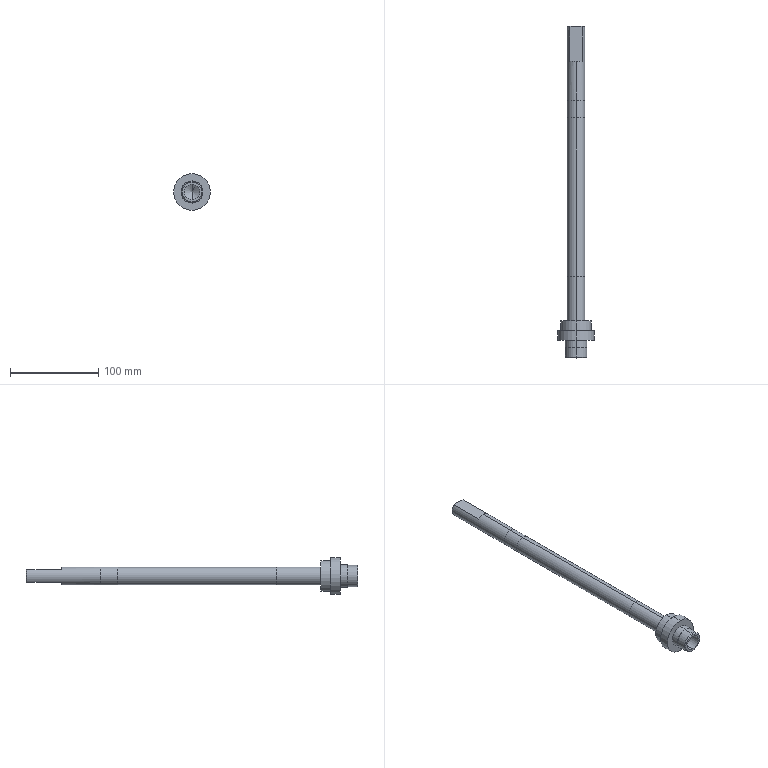Part | SolidWorks | features BaseBody 2 | 2 solids | 38 faces | box 41.4 x 376 x 41.4 mm | volume 127294 mm3 | cylinder 18 | plane 14 | cone 6 | commonest cylinder face diameters 20 x6 17.5 x2 19.8 x2 24 x2 25 x2 35 x2
STEP:
#1=CARTESIAN_POINT('',(7.141,244.,7.));
#2=VERTEX_POINT('',#1);
#3=CARTESIAN_POINT('',(0.,244.,10.));
#4=VERTEX_POINT('',#3);
#5=CARTESIAN_POINT('',(0.,244.,0.));
#6=DIRECTION('',(0.,-1.,0.));
#7=DIRECTION('',(0.,0.,-1.));
#8=AXIS2_PLACEMENT_3D('',#5,#6,#7);
#9=CIRCLE('',#8,10.);
#10=EDGE_CURVE('',#2,#4,#9,.T.);
#11=ORIENTED_EDGE('',*,*,#10,.T.);
#12=CARTESIAN_POINT('',(0.,200.,10.));
#13=VERTEX_POINT('',#12);
#14=CARTESIAN_POINT('',(0.,284.,10.));
#15=DIRECTION('',(0.,-1.,0.));
#16=VECTOR('',#15,1000.);
#17=LINE('',#14,#16);
#18=EDGE_CURVE('',#4,#13,#17,.T.);
#19=ORIENTED_EDGE('',*,*,#18,.T.);
#20=CARTESIAN_POINT('',(0.,200.,-10.));
#21=VERTEX_POINT('',#20);
#22=CARTESIAN_POINT('',(0.,200.,0.));
#23=DIRECTION('',(0.,1.,0.));
#24=DIRECTION('',(0.,0.,-1.));
#25=AXIS2_PLACEMENT_3D('',#22,#23,#24);
#26=CIRCLE('',#25,10.);
#27=EDGE_CURVE('',#13,#21,#26,.T.);
#28=ORIENTED_EDGE('',*,*,#27,.T.);
#29=CARTESIAN_POINT('',(0.,244.,-10.));
#30=VERTEX_POINT('',#29);
#31=CARTESIAN_POINT('',(0.,284.,-10.));
#32=DIRECTION('',(0.,-1.,0.));
#33=VECTOR('',#32,1000.);
#34=LINE('',#31,#33);
#35=EDGE_CURVE('',#30,#21,#34,.T.);
#36=ORIENTED_EDGE('',*,*,#35,.F.);
#37=CARTESIAN_POINT('',(7.141,244.,-7.));
#38=VERTEX_POINT('',#37);
#39=CARTESIAN_POINT('',(0.,244.,0.));
#40=DIRECTION('',(0.,-1.,0.));
#41=DIRECTION('',(0.,0.,-1.));
#42=AXIS2_PLACEMENT_3D('',#39,#40,#41);
#43=CIRCLE('',#42,10.);
#44=EDGE_CURVE('',#30,#38,#43,.T.);
#45=ORIENTED_EDGE('',*,*,#44,.T.);
#46=CARTESIAN_POINT('',(7.141,283.,-7.));
#47=VERTEX_POINT('',#46);
#48=CARTESIAN_POINT('',(7.141,284.,-7.));
#49=DIRECTION('',(0.,1.,0.));
#50=VECTOR('',#49,1000.);
#51=LINE('',#48,#50);
#52=EDGE_CURVE('',#38,#47,#51,.T.);
#53=ORIENTED_EDGE('',*,*,#52,.T.);
#54=CARTESIAN_POINT('',(7.141,283.,7.));
#55=VERTEX_POINT('',#54);
#56=CARTESIAN_POINT('',(0.,283.,0.));
#57=DIRECTION('',(0.,-1.,0.));
#58=DIRECTION('',(0.,0.,-1.));
#59=AXIS2_PLACEMENT_3D('',#56,#57,#58);
#60=CIRCLE('',#59,10.);
#61=EDGE_CURVE('',#47,#55,#60,.T.);
#62=ORIENTED_EDGE('',*,*,#61,.T.);
#63=CARTESIAN_POINT('',(7.141,284.,7.));
#64=DIRECTION('',(0.,-1.,0.));
#65=VECTOR('',#64,1000.);
#66=LINE('',#63,#65);
#67=EDGE_CURVE('',#55,#2,#66,.T.);
#68=ORIENTED_EDGE('',*,*,#67,.T.);
#69=EDGE_LOOP('',(#11,#19,#28,#36,#45,#53,#62,#68));
#70=FACE_OUTER_BOUND('',#69,.T.);
#71=CARTESIAN_POINT('',(0.,284.,0.));
#72=DIRECTION('',(0.,-1.,0.));
#73=DIRECTION('',(0.,0.,-1.));
#74=AXIS2_PLACEMENT_3D('',#71,#72,#73);
#75=CYLINDRICAL_SURFACE('',#74,10.);
#76=ADVANCED_FACE('',(#70),#75,.T.);
#77=ORIENTED_EDGE('',*,*,#18,.F.);
#78=CARTESIAN_POINT('',(-7.141,244.,7.));
#79=VERTEX_POINT('',#78);
#80=CARTESIAN_POINT('',(0.,244.,0.));
#81=DIRECTION('',(0.,-1.,0.));
#82=DIRECTION('',(0.,0.,-1.));
#83=AXIS2_PLACEMENT_3D('',#80,#81,#82);
#84=CIRCLE('',#83,10.);
#85=EDGE_CURVE('',#4,#79,#84,.T.);
#86=ORIENTED_EDGE('',*,*,#85,.T.);
#87=CARTESIAN_POINT('',(-7.141,283.,7.));
#88=VERTEX_POINT('',#87);
#89=CARTESIAN_POINT('',(-7.141,244.,7.));
#90=DIRECTION('',(0.,-1.,0.));
#91=VECTOR('',#90,1000.);
#92=LINE('',#89,#91);
#93=EDGE_CURVE('',#88,#79,#92,.T.);
#94=ORIENTED_EDGE('',*,*,#93,.F.);
#95=CARTESIAN_POINT('',(-7.141,283.,-7.));
#96=VERTEX_POINT('',#95);
#97=CARTESIAN_POINT('',(0.,283.,0.));
#98=DIRECTION('',(0.,-1.,0.));
#99=DIRECTION('',(0.,0.,-1.));
#100=AXIS2_PLACEMENT_3D('',#97,#98,#99);
#101=CIRCLE('',#100,10.);
#102=EDGE_CURVE('',#88,#96,#101,.T.);
#103=ORIENTED_EDGE('',*,*,#102,.T.);
#104=CARTESIAN_POINT('',(-7.141,244.,-7.));
#105=VERTEX_POINT('',#104);
#106=CARTESIAN_POINT('',(-7.141,244.,-7.));
#107=DIRECTION('',(0.,1.,0.));
#108=VECTOR('',#107,1000.);
#109=LINE('',#106,#108);
#110=EDGE_CURVE('',#105,#96,#109,.T.);
#111=ORIENTED_EDGE('',*,*,#110,.F.);
#112=CARTESIAN_POINT('',(0.,244.,0.));
#113=DIRECTION('',(0.,-1.,0.));
#114=DIRECTION('',(0.,0.,-1.));
#115=AXIS2_PLACEMENT_3D('',#112,#113,#114);
#116=CIRCLE('',#115,10.);
#117=EDGE_CURVE('',#105,#30,#116,.T.);
#118=ORIENTED_EDGE('',*,*,#117,.T.);
#119=ORIENTED_EDGE('',*,*,#35,.T.);
#120=CARTESIAN_POINT('',(0.,200.,0.));
#121=DIRECTION('',(0.,1.,0.));
#122=DIRECTION('',(0.,0.,-1.));
#123=AXIS2_PLACEMENT_3D('',#120,#121,#122);
#124=CIRCLE('',#123,10.);
#125=EDGE_CURVE('',#21,#13,#124,.T.);
#126=ORIENTED_EDGE('',*,*,#125,.T.);
#127=EDGE_LOOP('',(#77,#86,#94,#103,#111,#118,#119,#126));
#128=FACE_OUTER_BOUND('',#127,.T.);
#129=CARTESIAN_POINT('',(0.,284.,0.));
#130=DIRECTION('',(0.,-1.,0.));
#131=DIRECTION('',(0.,0.,-1.));
#132=AXIS2_PLACEMENT_3D('',#129,#130,#131);
#133=CYLINDRICAL_SURFACE('',#132,10.);
#134=ADVANCED_FACE('',(#128),#133,.T.);
#135=ORIENTED_EDGE('',*,*,#93,.T.);
#136=CARTESIAN_POINT('',(-15.568,244.,7.));
#137=DIRECTION('',(1.,0.,0.));
#138=VECTOR('',#137,1000.);
#139=LINE('',#136,#138);
#140=EDGE_CURVE('',#79,#2,#139,.T.);
#141=ORIENTED_EDGE('',*,*,#140,.T.);
#142=ORIENTED_EDGE('',*,*,#67,.F.);
#143=CARTESIAN_POINT('',(5.657,284.,7.));
#144=VERTEX_POINT('',#143);
#145=CARTESIAN_POINT('',(7.141,283.,7.));
#146=CARTESIAN_POINT('',(6.656,283.347,7.));
#147=CARTESIAN_POINT('',(6.162,283.682,7.));
#148=CARTESIAN_POINT('',(5.657,284.,7.));
#149=B_SPLINE_CURVE_WITH_KNOTS('',3,(#145,#146,#147,#148),.UNSPECIFIED.,.F.,.F.,(4,4),(0.,0.00179),.UNSPECIFIED.);
#150=EDGE_CURVE('',#55,#144,#149,.T.);
#151=ORIENTED_EDGE('',*,*,#150,.T.);
#152=CARTESIAN_POINT('',(-5.657,284.,7.));
#153=VERTEX_POINT('',#152);
#154=CARTESIAN_POINT('',(-15.568,284.,7.));
#155=DIRECTION('',(-1.,0.,0.));
#156=VECTOR('',#155,1000.);
#157=LINE('',#154,#156);
#158=EDGE_CURVE('',#144,#153,#157,.T.);
#159=ORIENTED_EDGE('',*,*,#158,.T.);
#160=CARTESIAN_POINT('',(-5.657,284.,7.));
#161=CARTESIAN_POINT('',(-6.162,283.682,7.));
#162=CARTESIAN_POINT('',(-6.656,283.347,7.));
#163=CARTESIAN_POINT('',(-7.141,283.,7.));
#164=B_SPLINE_CURVE_WITH_KNOTS('',3,(#160,#161,#162,#163),.UNSPECIFIED.,.F.,.F.,(4,4),(0.,0.00179),.UNSPECIFIED.);
#165=EDGE_CURVE('',#153,#88,#164,.T.);
#166=ORIENTED_EDGE('',*,*,#165,.T.);
#167=EDGE_LOOP('',(#135,#141,#142,#151,#159,#166));
#168=FACE_OUTER_BOUND('',#167,.T.);
#169=CARTESIAN_POINT('',(-15.568,244.,7.));
#170=DIRECTION('',(0.,0.,1.));
#171=DIRECTION('',(1.,0.,0.));
#172=AXIS2_PLACEMENT_3D('',#169,#170,#171);
#173=PLANE('',#172);
#174=ADVANCED_FACE('',(#168),#173,.T.);
#175=CARTESIAN_POINT('',(5.657,284.,-7.));
#176=VERTEX_POINT('',#175);
#177=CARTESIAN_POINT('',(7.141,283.,-7.));
#178=CARTESIAN_POINT('',(6.656,283.347,-7.));
#179=CARTESIAN_POINT('',(6.162,283.682,-7.));
#180=CARTESIAN_POINT('',(5.657,284.,-7.));
#181=B_SPLINE_CURVE_WITH_KNOTS('',3,(#177,#178,#179,#180),.UNSPECIFIED.,.F.,.F.,(4,4),(0.,0.00179),.UNSPECIFIED.);
#182=EDGE_CURVE('',#47,#176,#181,.T.);
#183=ORIENTED_EDGE('',*,*,#182,.T.);
#184=CARTESIAN_POINT('',(0.,284.,0.));
#185=DIRECTION('',(0.,-1.,0.));
#186=DIRECTION('',(0.,0.,-1.));
#187=AXIS2_PLACEMENT_3D('',#184,#185,#186);
#188=CIRCLE('',#187,9.);
#189=EDGE_CURVE('',#176,#144,#188,.T.);
#190=ORIENTED_EDGE('',*,*,#189,.T.);
#191=ORIENTED_EDGE('',*,*,#150,.F.);
#192=ORIENTED_EDGE('',*,*,#61,.F.);
#193=EDGE_LOOP('',(#183,#190,#191,#192));
#194=FACE_OUTER_BOUND('',#193,.T.);
#195=CARTESIAN_POINT('',(0.,283.,0.));
#196=DIRECTION('',(0.,-1.,0.));
#197=DIRECTION('',(0.,0.,-1.));
#198=AXIS2_PLACEMENT_3D('',#195,#196,#197);
#199=CONICAL_SURFACE('',#198,10.,0.7854);
#200=ADVANCED_FACE('',(#194),#199,.T.);
#201=ORIENTED_EDGE('',*,*,#110,.T.);
#202=CARTESIAN_POINT('',(-5.657,284.,-7.));
#203=VERTEX_POINT('',#202);
#204=CARTESIAN_POINT('',(-7.141,283.,-7.));
#205=CARTESIAN_POINT('',(-6.656,283.347,-7.));
#206=CARTESIAN_POINT('',(-6.162,283.682,-7.));
#207=CARTESIAN_POINT('',(-5.657,284.,-7.));
#208=B_SPLINE_CURVE_WITH_KNOTS('',3,(#204,#205,#206,#207),.UNSPECIFIED.,.F.,.F.,(4,4),(0.,0.00179),.UNSPECIFIED.);
#209=EDGE_CURVE('',#96,#203,#208,.T.);
#210=ORIENTED_EDGE('',*,*,#209,.T.);
#211=CARTESIAN_POINT('',(-15.568,284.,-7.));
#212=DIRECTION('',(1.,0.,0.));
#213=VECTOR('',#212,1000.);
#214=LINE('',#211,#213);
#215=EDGE_CURVE('',#203,#176,#214,.T.);
#216=ORIENTED_EDGE('',*,*,#215,.T.);
#217=ORIENTED_EDGE('',*,*,#182,.F.);
#218=ORIENTED_EDGE('',*,*,#52,.F.);
#219=CARTESIAN_POINT('',(-15.568,244.,-7.));
#220=DIRECTION('',(-1.,0.,0.));
#221=VECTOR('',#220,1000.);
#222=LINE('',#219,#221);
#223=EDGE_CURVE('',#38,#105,#222,.T.);
#224=ORIENTED_EDGE('',*,*,#223,.T.);
#225=EDGE_LOOP('',(#201,#210,#216,#217,#218,#224));
#226=FACE_OUTER_BOUND('',#225,.T.);
#227=CARTESIAN_POINT('',(-15.568,244.,-7.));
#228=DIRECTION('',(0.,0.,-1.));
#229=DIRECTION('',(-1.,0.,0.));
#230=AXIS2_PLACEMENT_3D('',#227,#228,#229);
#231=PLANE('',#230);
#232=ADVANCED_FACE('',(#226),#231,.T.);
#233=ORIENTED_EDGE('',*,*,#117,.F.);
#234=ORIENTED_EDGE('',*,*,#223,.F.);
#235=ORIENTED_EDGE('',*,*,#44,.F.);
#236=EDGE_LOOP('',(#233,#234,#235));
#237=FACE_OUTER_BOUND('',#236,.T.);
#238=CARTESIAN_POINT('',(0.,244.,0.));
#239=DIRECTION('',(0.,1.,0.));
#240=DIRECTION('',(0.,0.,1.));
#241=AXIS2_PLACEMENT_3D('',#238,#239,#240);
#242=PLANE('',#241);
#243=ADVANCED_FACE('',(#237),#242,.T.);
#244=ORIENTED_EDGE('',*,*,#125,.F.);
#245=ORIENTED_EDGE('',*,*,#27,.F.);
#246=EDGE_LOOP('',(#244,#245));
#247=FACE_OUTER_BOUND('',#246,.T.);
#248=CARTESIAN_POINT('',(0.,200.,0.));
#249=DIRECTION('',(0.,1.,0.));
#250=DIRECTION('',(0.,0.,1.));
#251=AXIS2_PLACEMENT_3D('',#248,#249,#250);
#252=PLANE('',#251);
#253=ADVANCED_FACE('',(#247),#252,.F.);
#254=ORIENTED_EDGE('',*,*,#10,.F.);
#255=ORIENTED_EDGE('',*,*,#140,.F.);
#256=ORIENTED_EDGE('',*,*,#85,.F.);
#257=EDGE_LOOP('',(#254,#255,#256));
#258=FACE_OUTER_BOUND('',#257,.T.);
#259=CARTESIAN_POINT('',(0.,244.,0.));
#260=DIRECTION('',(0.,1.,0.));
#261=DIRECTION('',(0.,0.,1.));
#262=AXIS2_PLACEMENT_3D('',#259,#260,#261);
#263=PLANE('',#262);
#264=ADVANCED_FACE('',(#258),#263,.T.);
#265=ORIENTED_EDGE('',*,*,#165,.F.);
#266=CARTESIAN_POINT('',(0.,284.,0.));
#267=DIRECTION('',(0.,-1.,0.));
#268=DIRECTION('',(0.,0.,-1.));
#269=AXIS2_PLACEMENT_3D('',#266,#267,#268);
#270=CIRCLE('',#269,9.);
#271=EDGE_CURVE('',#153,#203,#270,.T.);
#272=ORIENTED_EDGE('',*,*,#271,.T.);
#273=ORIENTED_EDGE('',*,*,#209,.F.);
#274=ORIENTED_EDGE('',*,*,#102,.F.);
#275=EDGE_LOOP('',(#265,#272,#273,#274));
#276=FACE_OUTER_BOUND('',#275,.T.);
#277=CARTESIAN_POINT('',(0.,283.,0.));
#278=DIRECTION('',(0.,-1.,0.));
#279=DIRECTION('',(0.,0.,-1.));
#280=AXIS2_PLACEMENT_3D('',#277,#278,#279);
#281=CONICAL_SURFACE('',#280,10.,0.7854);
#282=ADVANCED_FACE('',(#276),#281,.T.);
#283=ORIENTED_EDGE('',*,*,#215,.F.);
#284=ORIENTED_EDGE('',*,*,#271,.F.);
#285=ORIENTED_EDGE('',*,*,#158,.F.);
#286=ORIENTED_EDGE('',*,*,#189,.F.);
#287=EDGE_LOOP('',(#283,#284,#285,#286));
#288=FACE_OUTER_BOUND('',#287,.T.);
#289=CARTESIAN_POINT('',(0.,284.,0.));
#290=DIRECTION('',(0.,1.,0.));
#291=DIRECTION('',(0.,0.,1.));
#292=AXIS2_PLACEMENT_3D('',#289,#290,#291);
#293=PLANE('',#292);
#294=ADVANCED_FACE('',(#288),#293,.T.);
#295=CLOSED_SHELL('',(#76,#134,#174,#200,#232,#243,#253,#264,#282,#294));
#296=MANIFOLD_SOLID_BREP('',#295);
#297=CARTESIAN_POINT('',(0.,180.,-9.9));
#298=VERTEX_POINT('',#297);
#299=CARTESIAN_POINT('',(0.,180.,9.9));
#300=VERTEX_POINT('',#299);
#301=CARTESIAN_POINT('',(0.,180.,0.));
#302=DIRECTION('',(0.,-1.,0.));
#303=DIRECTION('',(0.,0.,-1.));
#304=AXIS2_PLACEMENT_3D('',#301,#302,#303);
#305=CIRCLE('',#304,9.9);
#306=EDGE_CURVE('',#298,#300,#305,.T.);
#307=ORIENTED_EDGE('',*,*,#306,.T.);
#308=CARTESIAN_POINT('',(0.,0.,9.9));
#309=VERTEX_POINT('',#308);
#310=CARTESIAN_POINT('',(0.,180.,9.9));
#311=DIRECTION('',(0.,-1.,0.));
#312=VECTOR('',#311,1000.);
#313=LINE('',#310,#312);
#314=EDGE_CURVE('',#300,#309,#313,.T.);
#315=ORIENTED_EDGE('',*,*,#314,.T.);
#316=CARTESIAN_POINT('',(0.,0.,-9.9));
#317=VERTEX_POINT('',#316);
#318=CARTESIAN_POINT('',(0.,0.,0.));
#319=DIRECTION('',(0.,1.,0.));
#320=DIRECTION('',(0.,0.,-1.));
#321=AXIS2_PLACEMENT_3D('',#318,#319,#320);
#322=CIRCLE('',#321,9.9);
#323=EDGE_CURVE('',#309,#317,#322,.T.);
#324=ORIENTED_EDGE('',*,*,#323,.T.);
#325=CARTESIAN_POINT('',(0.,180.,-9.9));
#326=DIRECTION('',(0.,-1.,0.));
#327=VECTOR('',#326,1000.);
#328=LINE('',#325,#327);
#329=EDGE_CURVE('',#298,#317,#328,.T.);
#330=ORIENTED_EDGE('',*,*,#329,.F.);
#331=EDGE_LOOP('',(#307,#315,#324,#330));
#332=FACE_OUTER_BOUND('',#331,.T.);
#333=CARTESIAN_POINT('',(0.,180.,0.));
#334=DIRECTION('',(0.,-1.,0.));
#335=DIRECTION('',(0.,0.,-1.));
#336=AXIS2_PLACEMENT_3D('',#333,#334,#335);
#337=CYLINDRICAL_SURFACE('',#336,9.9);
#338=ADVANCED_FACE('',(#332),#337,.T.);
#339=CARTESIAN_POINT('',(0.,-50.,10.));
#340=VERTEX_POINT('',#339);
#341=CARTESIAN_POINT('',(0.,-50.,-10.));
#342=VERTEX_POINT('',#341);
#343=CARTESIAN_POINT('',(0.,-50.,0.));
#344=DIRECTION('',(0.,1.,0.));
#345=DIRECTION('',(0.,0.,1.));
#346=AXIS2_PLACEMENT_3D('',#343,#344,#345);
#347=CIRCLE('',#346,10.);
#348=EDGE_CURVE('',#340,#342,#347,.T.);
#349=ORIENTED_EDGE('',*,*,#348,.T.);
#350=CARTESIAN_POINT('',(0.,0.,-10.));
#351=VERTEX_POINT('',#350);
#352=CARTESIAN_POINT('',(0.,-50.,-10.));
#353=DIRECTION('',(0.,1.,0.));
#354=VECTOR('',#353,1000.);
#355=LINE('',#352,#354);
#356=EDGE_CURVE('',#342,#351,#355,.T.);
#357=ORIENTED_EDGE('',*,*,#356,.T.);
#358=CARTESIAN_POINT('',(0.,0.,10.));
#359=VERTEX_POINT('',#358);
#360=CARTESIAN_POINT('',(0.,0.,0.));
#361=DIRECTION('',(0.,-1.,0.));
#362=DIRECTION('',(0.,0.,1.));
#363=AXIS2_PLACEMENT_3D('',#360,#361,#362);
#364=CIRCLE('',#363,10.);
#365=EDGE_CURVE('',#351,#359,#364,.T.);
#366=ORIENTED_EDGE('',*,*,#365,.T.);
#367=CARTESIAN_POINT('',(0.,-50.,10.));
#368=DIRECTION('',(0.,1.,0.));
#369=VECTOR('',#368,1000.);
#370=LINE('',#367,#369);
#371=EDGE_CURVE('',#340,#359,#370,.T.);
#372=ORIENTED_EDGE('',*,*,#371,.F.);
#373=EDGE_LOOP('',(#349,#357,#366,#372));
#374=FACE_OUTER_BOUND('',#373,.T.);
#375=CARTESIAN_POINT('',(0.,-50.,0.));
#376=DIRECTION('',(0.,1.,0.));
#377=DIRECTION('',(0.,0.,1.));
#378=AXIS2_PLACEMENT_3D('',#375,#376,#377);
#379=CYLINDRICAL_SURFACE('',#378,10.);
#380=ADVANCED_FACE('',(#374),#379,.T.);
#381=CARTESIAN_POINT('',(0.,200.,-10.));
#382=VERTEX_POINT('',#381);
#383=CARTESIAN_POINT('',(0.,200.,10.));
#384=VERTEX_POINT('',#383);
#385=CARTESIAN_POINT('',(0.,200.,0.));
#386=DIRECTION('',(0.,-1.,0.));
#387=DIRECTION('',(0.,0.,-1.));
#388=AXIS2_PLACEMENT_3D('',#385,#386,#387);
#389=CIRCLE('',#388,10.);
#390=EDGE_CURVE('',#382,#384,#389,.T.);
#391=ORIENTED_EDGE('',*,*,#390,.T.);
#392=CARTESIAN_POINT('',(0.,180.,10.));
#393=VERTEX_POINT('',#392);
#394=CARTESIAN_POINT('',(0.,200.,10.));
#395=DIRECTION('',(0.,-1.,0.));
#396=VECTOR('',#395,1000.);
#397=LINE('',#394,#396);
#398=EDGE_CURVE('',#384,#393,#397,.T.);
#399=ORIENTED_EDGE('',*,*,#398,.T.);
#400=CARTESIAN_POINT('',(0.,180.,-10.));
#401=VERTEX_POINT('',#400);
#402=CARTESIAN_POINT('',(0.,180.,0.));
#403=DIRECTION('',(0.,1.,0.));
#404=DIRECTION('',(0.,0.,-1.));
#405=AXIS2_PLACEMENT_3D('',#402,#403,#404);
#406=CIRCLE('',#405,10.);
#407=EDGE_CURVE('',#393,#401,#406,.T.);
#408=ORIENTED_EDGE('',*,*,#407,.T.);
#409=CARTESIAN_POINT('',(0.,200.,-10.));
#410=DIRECTION('',(0.,-1.,0.));
#411=VECTOR('',#410,1000.);
#412=LINE('',#409,#411);
#413=EDGE_CURVE('',#382,#401,#412,.T.);
#414=ORIENTED_EDGE('',*,*,#413,.F.);
#415=EDGE_LOOP('',(#391,#399,#408,#414));
#416=FACE_OUTER_BOUND('',#415,.T.);
#417=CARTESIAN_POINT('',(0.,200.,0.));
#418=DIRECTION('',(0.,-1.,0.));
#419=DIRECTION('',(0.,0.,-1.));
#420=AXIS2_PLACEMENT_3D('',#417,#418,#419);
#421=CYLINDRICAL_SURFACE('',#420,10.);
#422=ADVANCED_FACE('',(#416),#421,.T.);
#423=CARTESIAN_POINT('',(0.,-61.,17.5));
#424=VERTEX_POINT('',#423);
#425=CARTESIAN_POINT('',(0.,-61.,-17.5));
#426=VERTEX_POINT('',#425);
#427=CARTESIAN_POINT('',(0.,-61.,0.));
#428=DIRECTION('',(0.,1.,0.));
#429=DIRECTION('',(0.,0.,1.));
#430=AXIS2_PLACEMENT_3D('',#427,#428,#429);
#431=CIRCLE('',#430,17.5);
#432=EDGE_CURVE('',#424,#426,#431,.T.);
#433=ORIENTED_EDGE('',*,*,#432,.T.);
#434=CARTESIAN_POINT('',(0.,-50.,-17.5));
#435=VERTEX_POINT('',#434);
#436=CARTESIAN_POINT('',(0.,-61.,-17.5));
#437=DIRECTION('',(0.,1.,0.));
#438=VECTOR('',#437,1000.);
#439=LINE('',#436,#438);
#440=EDGE_CURVE('',#426,#435,#439,.T.);
#441=ORIENTED_EDGE('',*,*,#440,.T.);
#442=CARTESIAN_POINT('',(0.,-50.,17.5));
#443=VERTEX_POINT('',#442);
#444=CARTESIAN_POINT('',(0.,-50.,0.));
#445=DIRECTION('',(0.,-1.,0.));
#446=DIRECTION('',(0.,0.,1.));
#447=AXIS2_PLACEMENT_3D('',#444,#445,#446);
#448=CIRCLE('',#447,17.5);
#449=EDGE_CURVE('',#435,#443,#448,.T.);
#450=ORIENTED_EDGE('',*,*,#449,.T.);
#451=CARTESIAN_POINT('',(0.,-61.,17.5));
#452=DIRECTION('',(0.,1.,0.));
#453=VECTOR('',#452,1000.);
#454=LINE('',#451,#453);
#455=EDGE_CURVE('',#424,#443,#454,.T.);
#456=ORIENTED_EDGE('',*,*,#455,.F.);
#457=EDGE_LOOP('',(#433,#441,#450,#456));
#458=FACE_OUTER_BOUND('',#457,.T.);
#459=CARTESIAN_POINT('',(0.,-61.,0.));
#460=DIRECTION('',(0.,1.,0.));
#461=DIRECTION('',(0.,0.,1.));
#462=AXIS2_PLACEMENT_3D('',#459,#460,#461);
#463=CYLINDRICAL_SURFACE('',#462,17.5);
#464=ADVANCED_FACE('',(#458),#463,.T.);
#465=CARTESIAN_POINT('',(0.,-72.,20.7));
#466=VERTEX_POINT('',#465);
#467=CARTESIAN_POINT('',(0.,-72.,-20.7));
#468=VERTEX_POINT('',#467);
#469=CARTESIAN_POINT('',(0.,-72.,0.));
#470=DIRECTION('',(0.,1.,0.));
#471=DIRECTION('',(0.,0.,1.));
#472=AXIS2_PLACEMENT_3D('',#469,#470,#471);
#473=CIRCLE('',#472,20.7);
#474=EDGE_CURVE('',#466,#468,#473,.T.);
#475=ORIENTED_EDGE('',*,*,#474,.T.);
#476=CARTESIAN_POINT('',(0.,-61.,-20.7));
#477=VERTEX_POINT('',#476);
#478=CARTESIAN_POINT('',(0.,-72.,-20.7));
#479=DIRECTION('',(0.,1.,0.));
#480=VECTOR('',#479,1000.);
#481=LINE('',#478,#480);
#482=EDGE_CURVE('',#468,#477,#481,.T.);
#483=ORIENTED_EDGE('',*,*,#482,.T.);
#484=CARTESIAN_POINT('',(0.,-61.,20.7));
#485=VERTEX_POINT('',#484);
#486=CARTESIAN_POINT('',(0.,-61.,0.));
#487=DIRECTION('',(0.,-1.,0.));
#488=DIRECTION('',(0.,0.,1.));
#489=AXIS2_PLACEMENT_3D('',#486,#487,#488);
#490=CIRCLE('',#489,20.7);
#491=EDGE_CURVE('',#477,#485,#490,.T.);
#492=ORIENTED_EDGE('',*,*,#491,.T.);
#493=CARTESIAN_POINT('',(0.,-72.,20.7));
#494=DIRECTION('',(0.,1.,0.));
#495=VECTOR('',#494,1000.);
#496=LINE('',#493,#495);
#497=EDGE_CURVE('',#466,#485,#496,.T.);
#498=ORIENTED_EDGE('',*,*,#497,.F.);
#499=EDGE_LOOP('',(#475,#483,#492,#498));
#500=FACE_OUTER_BOUND('',#499,.T.);
#501=CARTESIAN_POINT('',(0.,-72.,0.));
#502=DIRECTION('',(0.,1.,0.));
#503=DIRECTION('',(0.,0.,1.));
#504=AXIS2_PLACEMENT_3D('',#501,#502,#503);
#505=CYLINDRICAL_SURFACE('',#504,20.7);
#506=ADVANCED_FACE('',(#500),#505,.T.);
#507=CARTESIAN_POINT('',(0.,-80.,12.5));
#508=VERTEX_POINT('',#507);
#509=CARTESIAN_POINT('',(0.,-80.,-12.5));
#510=VERTEX_POINT('',#509);
#511=CARTESIAN_POINT('',(0.,-80.,0.));
#512=DIRECTION('',(0.,1.,0.));
#513=DIRECTION('',(0.,0.,1.));
#514=AXIS2_PLACEMENT_3D('',#511,#512,#513);
#515=CIRCLE('',#514,12.5);
#516=EDGE_CURVE('',#508,#510,#515,.T.);
#517=ORIENTED_EDGE('',*,*,#516,.T.);
#518=CARTESIAN_POINT('',(0.,-72.,-12.5));
#519=VERTEX_POINT('',#518);
#520=CARTESIAN_POINT('',(0.,-80.,-12.5));
#521=DIRECTION('',(0.,1.,0.));
#522=VECTOR('',#521,1000.);
#523=LINE('',#520,#522);
#524=EDGE_CURVE('',#510,#519,#523,.T.);
#525=ORIENTED_EDGE('',*,*,#524,.T.);
#526=CARTESIAN_POINT('',(0.,-72.,12.5));
#527=VERTEX_POINT('',#526);
#528=CARTESIAN_POINT('',(0.,-72.,0.));
#529=DIRECTION('',(0.,1.,0.));
#530=DIRECTION('',(0.,0.,1.));
#531=AXIS2_PLACEMENT_3D('',#528,#529,#530);
#532=CIRCLE('',#531,12.5);
#533=EDGE_CURVE('',#527,#519,#532,.T.);
#534=ORIENTED_EDGE('',*,*,#533,.F.);
#535=CARTESIAN_POINT('',(0.,-80.,12.5));
#536=DIRECTION('',(0.,1.,0.));
#537=VECTOR('',#536,1000.);
#538=LINE('',#535,#537);
#539=EDGE_CURVE('',#508,#527,#538,.T.);
#540=ORIENTED_EDGE('',*,*,#539,.F.);
#541=EDGE_LOOP('',(#517,#525,#534,#540));
#542=FACE_OUTER_BOUND('',#541,.T.);
#543=CARTESIAN_POINT('',(0.,-80.,0.));
#544=DIRECTION('',(0.,1.,0.));
#545=DIRECTION('',(0.,0.,1.));
#546=AXIS2_PLACEMENT_3D('',#543,#544,#545);
#547=CYLINDRICAL_SURFACE('',#546,12.5);
#548=ADVANCED_FACE('',(#542),#547,.T.);
#549=CARTESIAN_POINT('',(0.,-91.,12.));
#550=VERTEX_POINT('',#549);
#551=CARTESIAN_POINT('',(0.,-91.,-12.));
#552=VERTEX_POINT('',#551);
#553=CARTESIAN_POINT('',(0.,-91.,0.));
#554=DIRECTION('',(0.,1.,0.));
#555=DIRECTION('',(0.,0.,1.));
#556=AXIS2_PLACEMENT_3D('',#553,#554,#555);
#557=CIRCLE('',#556,12.);
#558=EDGE_CURVE('',#550,#552,#557,.T.);
#559=ORIENTED_EDGE('',*,*,#558,.T.);
#560=CARTESIAN_POINT('',(0.,-80.,-12.));
#561=VERTEX_POINT('',#560);
#562=CARTESIAN_POINT('',(0.,-92.,-12.));
#563=DIRECTION('',(0.,1.,0.));
#564=VECTOR('',#563,1000.);
#565=LINE('',#562,#564);
#566=EDGE_CURVE('',#552,#561,#565,.T.);
#567=ORIENTED_EDGE('',*,*,#566,.T.);
#568=CARTESIAN_POINT('',(0.,-80.,12.));
#569=VERTEX_POINT('',#568);
#570=CARTESIAN_POINT('',(0.,-80.,0.));
#571=DIRECTION('',(0.,1.,0.));
#572=DIRECTION('',(0.,0.,1.));
#573=AXIS2_PLACEMENT_3D('',#570,#571,#572);
#574=CIRCLE('',#573,12.);
#575=EDGE_CURVE('',#569,#561,#574,.T.);
#576=ORIENTED_EDGE('',*,*,#575,.F.);
#577=CARTESIAN_POINT('',(0.,-92.,12.));
#578=DIRECTION('',(0.,1.,0.));
#579=VECTOR('',#578,1000.);
#580=LINE('',#577,#579);
#581=EDGE_CURVE('',#550,#569,#580,.T.);
#582=ORIENTED_EDGE('',*,*,#581,.F.);
#583=EDGE_LOOP('',(#559,#567,#576,#582));
#584=FACE_OUTER_BOUND('',#583,.T.);
#585=CARTESIAN_POINT('',(0.,-92.,0.));
#586=DIRECTION('',(0.,1.,0.));
#587=DIRECTION('',(0.,0.,1.));
#588=AXIS2_PLACEMENT_3D('',#585,#586,#587);
#589=CYLINDRICAL_SURFACE('',#588,12.);
#590=ADVANCED_FACE('',(#584),#589,.T.);
#591=CARTESIAN_POINT('',(0.,-92.,11.));
#592=VERTEX_POINT('',#591);
#593=CARTESIAN_POINT('',(0.,-92.,-11.));
#594=VERTEX_POINT('',#593);
#595=CARTESIAN_POINT('',(0.,-92.,0.));
#596=DIRECTION('',(0.,1.,0.));
#597=DIRECTION('',(0.,0.,1.));
#598=AXIS2_PLACEMENT_3D('',#595,#596,#597);
#599=CIRCLE('',#598,11.);
#600=EDGE_CURVE('',#592,#594,#599,.T.);
#601=ORIENTED_EDGE('',*,*,#600,.T.);
#602=CARTESIAN_POINT('',(0.,-91.,-12.));
#603=DIRECTION('',(0.,0.7071,-0.7071));
#604=VECTOR('',#603,1000.);
#605=LINE('',#602,#604);
#606=EDGE_CURVE('',#594,#552,#605,.T.);
#607=ORIENTED_EDGE('',*,*,#606,.T.);
#608=ORIENTED_EDGE('',*,*,#558,.F.);
#609=CARTESIAN_POINT('',(0.,-91.,12.));
#610=DIRECTION('',(0.,0.7071,0.7071));
#611=VECTOR('',#610,1000.);
#612=LINE('',#609,#611);
#613=EDGE_CURVE('',#592,#550,#612,.T.);
#614=ORIENTED_EDGE('',*,*,#613,.F.);
#615=EDGE_LOOP('',(#601,#607,#608,#614));
#616=FACE_OUTER_BOUND('',#615,.T.);
#617=CARTESIAN_POINT('',(0.,-91.,0.));
#618=DIRECTION('',(0.,1.,0.));
#619=DIRECTION('',(0.,0.,1.));
#620=AXIS2_PLACEMENT_3D('',#617,#618,#619);
#621=CONICAL_SURFACE('',#620,12.,0.7854);
#622=ADVANCED_FACE('',(#616),#621,.T.);
#623=CARTESIAN_POINT('',(0.,-57.,8.75));
#624=VERTEX_POINT('',#623);
#625=CARTESIAN_POINT('',(0.,-57.,-8.75));
#626=VERTEX_POINT('',#625);
#627=CARTESIAN_POINT('',(0.,-57.,0.));
#628=DIRECTION('',(0.,-1.,0.));
#629=DIRECTION('',(0.,0.,-1.));
#630=AXIS2_PLACEMENT_3D('',#627,#628,#629);
#631=CIRCLE('',#630,8.75);
#632=EDGE_CURVE('',#624,#626,#631,.T.);
#633=ORIENTED_EDGE('',*,*,#632,.F.);
#634=CARTESIAN_POINT('',(0.,-92.,8.75));
#635=VERTEX_POINT('',#634);
#636=CARTESIAN_POINT('',(0.,-92.,8.75));
#637=DIRECTION('',(0.,-1.,0.));
#638=VECTOR('',#637,1000.);
#639=LINE('',#636,#638);
#640=EDGE_CURVE('',#624,#635,#639,.T.);
#641=ORIENTED_EDGE('',*,*,#640,.T.);
#642=CARTESIAN_POINT('',(0.,-92.,-8.75));
#643=VERTEX_POINT('',#642);
#644=CARTESIAN_POINT('',(0.,-92.,0.));
#645=DIRECTION('',(0.,1.,0.));
#646=DIRECTION('',(0.,0.,-1.));
#647=AXIS2_PLACEMENT_3D('',#644,#645,#646);
#648=CIRCLE('',#647,8.75);
#649=EDGE_CURVE('',#643,#635,#648,.T.);
#650=ORIENTED_EDGE('',*,*,#649,.F.);
#651=CARTESIAN_POINT('',(0.,-92.,-8.75));
#652=DIRECTION('',(0.,-1.,0.));
#653=VECTOR('',#652,1000.);
#654=LINE('',#651,#653);
#655=EDGE_CURVE('',#626,#643,#654,.T.);
#656=ORIENTED_EDGE('',*,*,#655,.F.);
#657=EDGE_LOOP('',(#633,#641,#650,#656));
#658=FACE_OUTER_BOUND('',#657,.T.);
#659=CARTESIAN_POINT('',(0.,-92.,0.));
#660=DIRECTION('',(0.,-1.,0.));
#661=DIRECTION('',(0.,0.,-1.));
#662=AXIS2_PLACEMENT_3D('',#659,#660,#661);
#663=CYLINDRICAL_SURFACE('',#662,8.75);
#664=ADVANCED_FACE('',(#658),#663,.F.);
#665=CARTESIAN_POINT('',(0.,-51.742,0.));
#666=VERTEX_POINT('',#665);
#667=CARTESIAN_POINT('',(0.,-57.,-8.75));
#668=DIRECTION('',(0.,-0.515,-0.8572));
#669=VECTOR('',#668,1000.);
#670=LINE('',#667,#669);
#671=EDGE_CURVE('',#666,#626,#670,.T.);
#672=ORIENTED_EDGE('',*,*,#671,.F.);
#673=CARTESIAN_POINT('',(0.,-57.,8.75));
#674=DIRECTION('',(0.,-0.515,0.8572));
#675=VECTOR('',#674,1000.);
#676=LINE('',#673,#675);
#677=EDGE_CURVE('',#666,#624,#676,.T.);
#678=ORIENTED_EDGE('',*,*,#677,.T.);
#679=ORIENTED_EDGE('',*,*,#632,.T.);
#680=EDGE_LOOP('',(#672,#678,#679));
#681=FACE_OUTER_BOUND('',#680,.T.);
#682=CARTESIAN_POINT('',(0.,-57.,0.));
#683=DIRECTION('',(0.,-1.,0.));
#684=DIRECTION('',(0.,0.,-1.));
#685=AXIS2_PLACEMENT_3D('',#682,#683,#684);
#686=CONICAL_SURFACE('',#685,8.75,1.03);
#687=ADVANCED_FACE('',(#681),#686,.F.);
#688=ORIENTED_EDGE('',*,*,#314,.F.);
#689=CARTESIAN_POINT('',(0.,180.,0.));
#690=DIRECTION('',(0.,-1.,0.));
#691=DIRECTION('',(0.,0.,-1.));
#692=AXIS2_PLACEMENT_3D('',#689,#690,#691);
#693=CIRCLE('',#692,9.9);
#694=EDGE_CURVE('',#300,#298,#693,.T.);
#695=ORIENTED_EDGE('',*,*,#694,.T.);
#696=ORIENTED_EDGE('',*,*,#329,.T.);
#697=CARTESIAN_POINT('',(0.,0.,0.));
#698=DIRECTION('',(0.,1.,0.));
#699=DIRECTION('',(0.,0.,-1.));
#700=AXIS2_PLACEMENT_3D('',#697,#698,#699);
#701=CIRCLE('',#700,9.9);
#702=EDGE_CURVE('',#317,#309,#701,.T.);
#703=ORIENTED_EDGE('',*,*,#702,.T.);
#704=EDGE_LOOP('',(#688,#695,#696,#703));
#705=FACE_OUTER_BOUND('',#704,.T.);
#706=CARTESIAN_POINT('',(0.,180.,0.));
#707=DIRECTION('',(0.,-1.,0.));
#708=DIRECTION('',(0.,0.,-1.));
#709=AXIS2_PLACEMENT_3D('',#706,#707,#708);
#710=CYLINDRICAL_SURFACE('',#709,9.9);
#711=ADVANCED_FACE('',(#705),#710,.T.);
#712=CARTESIAN_POINT('',(0.,0.,0.));
#713=DIRECTION('',(0.,-1.,0.));
#714=DIRECTION('',(0.,0.,1.));
#715=AXIS2_PLACEMENT_3D('',#712,#713,#714);
#716=CIRCLE('',#715,10.);
#717=EDGE_CURVE('',#359,#351,#716,.T.);
#718=ORIENTED_EDGE('',*,*,#717,.F.);
#719=ORIENTED_EDGE('',*,*,#365,.F.);
#720=EDGE_LOOP('',(#718,#719));
#721=FACE_OUTER_BOUND('',#720,.T.);
#722=ORIENTED_EDGE('',*,*,#702,.F.);
#723=ORIENTED_EDGE('',*,*,#323,.F.);
#724=EDGE_LOOP('',(#722,#723));
#725=FACE_BOUND('',#724,.T.);
#726=CARTESIAN_POINT('',(0.,0.,0.));
#727=DIRECTION('',(0.,-1.,0.));
#728=DIRECTION('',(0.,0.,-1.));
#729=AXIS2_PLACEMENT_3D('',#726,#727,#728);
#730=PLANE('',#729);
#731=ADVANCED_FACE('',(#721,#725),#730,.F.);
#732=CARTESIAN_POINT('',(0.,180.,0.));
#733=DIRECTION('',(0.,1.,0.));
#734=DIRECTION('',(0.,0.,-1.));
#735=AXIS2_PLACEMENT_3D('',#732,#733,#734);
#736=CIRCLE('',#735,10.);
#737=EDGE_CURVE('',#401,#393,#736,.T.);
#738=ORIENTED_EDGE('',*,*,#737,.F.);
#739=ORIENTED_EDGE('',*,*,#407,.F.);
#740=EDGE_LOOP('',(#738,#739));
#741=FACE_OUTER_BOUND('',#740,.T.);
#742=ORIENTED_EDGE('',*,*,#306,.F.);
#743=ORIENTED_EDGE('',*,*,#694,.F.);
#744=EDGE_LOOP('',(#742,#743));
#745=FACE_BOUND('',#744,.T.);
#746=CARTESIAN_POINT('',(0.,180.,0.));
#747=DIRECTION('',(0.,1.,0.));
#748=DIRECTION('',(0.,0.,1.));
#749=AXIS2_PLACEMENT_3D('',#746,#747,#748);
#750=PLANE('',#749);
#751=ADVANCED_FACE('',(#741,#745),#750,.F.);
#752=ORIENTED_EDGE('',*,*,#356,.F.);
#753=CARTESIAN_POINT('',(0.,-50.,0.));
#754=DIRECTION('',(0.,1.,0.));
#755=DIRECTION('',(0.,0.,1.));
#756=AXIS2_PLACEMENT_3D('',#753,#754,#755);
#757=CIRCLE('',#756,10.);
#758=EDGE_CURVE('',#342,#340,#757,.T.);
#759=ORIENTED_EDGE('',*,*,#758,.T.);
#760=ORIENTED_EDGE('',*,*,#371,.T.);
#761=ORIENTED_EDGE('',*,*,#717,.T.);
#762=EDGE_LOOP('',(#752,#759,#760,#761));
#763=FACE_OUTER_BOUND('',#762,.T.);
#764=CARTESIAN_POINT('',(0.,-50.,0.));
#765=DIRECTION('',(0.,1.,0.));
#766=DIRECTION('',(0.,0.,1.));
#767=AXIS2_PLACEMENT_3D('',#764,#765,#766);
#768=CYLINDRICAL_SURFACE('',#767,10.);
#769=ADVANCED_FACE('',(#763),#768,.T.);
#770=ORIENTED_EDGE('',*,*,#398,.F.);
#771=CARTESIAN_POINT('',(0.,200.,0.));
#772=DIRECTION('',(0.,-1.,0.));
#773=DIRECTION('',(0.,0.,-1.));
#774=AXIS2_PLACEMENT_3D('',#771,#772,#773);
#775=CIRCLE('',#774,10.);
#776=EDGE_CURVE('',#384,#382,#775,.T.);
#777=ORIENTED_EDGE('',*,*,#776,.T.);
#778=ORIENTED_EDGE('',*,*,#413,.T.);
#779=ORIENTED_EDGE('',*,*,#737,.T.);
#780=EDGE_LOOP('',(#770,#777,#778,#779));
#781=FACE_OUTER_BOUND('',#780,.T.);
#782=CARTESIAN_POINT('',(0.,200.,0.));
#783=DIRECTION('',(0.,-1.,0.));
#784=DIRECTION('',(0.,0.,-1.));
#785=AXIS2_PLACEMENT_3D('',#782,#783,#784);
#786=CYLINDRICAL_SURFACE('',#785,10.);
#787=ADVANCED_FACE('',(#781),#786,.T.);
#788=CARTESIAN_POINT('',(0.,-50.,0.));
#789=DIRECTION('',(0.,-1.,0.));
#790=DIRECTION('',(0.,0.,1.));
#791=AXIS2_PLACEMENT_3D('',#788,#789,#790);
#792=CIRCLE('',#791,17.5);
#793=EDGE_CURVE('',#443,#435,#792,.T.);
#794=ORIENTED_EDGE('',*,*,#793,.F.);
#795=ORIENTED_EDGE('',*,*,#449,.F.);
#796=EDGE_LOOP('',(#794,#795));
#797=FACE_OUTER_BOUND('',#796,.T.);
#798=ORIENTED_EDGE('',*,*,#348,.F.);
#799=ORIENTED_EDGE('',*,*,#758,.F.);
#800=EDGE_LOOP('',(#798,#799));
#801=FACE_BOUND('',#800,.T.);
#802=CARTESIAN_POINT('',(0.,-50.,0.));
#803=DIRECTION('',(0.,-1.,0.));
#804=DIRECTION('',(0.,0.,-1.));
#805=AXIS2_PLACEMENT_3D('',#802,#803,#804);
#806=PLANE('',#805);
#807=ADVANCED_FACE('',(#797,#801),#806,.F.);
#808=ORIENTED_EDGE('',*,*,#390,.F.);
#809=ORIENTED_EDGE('',*,*,#776,.F.);
#810=EDGE_LOOP('',(#808,#809));
#811=FACE_OUTER_BOUND('',#810,.T.);
#812=CARTESIAN_POINT('',(0.,200.,0.));
#813=DIRECTION('',(0.,1.,0.));
#814=DIRECTION('',(0.,0.,1.));
#815=AXIS2_PLACEMENT_3D('',#812,#813,#814);
#816=PLANE('',#815);
#817=ADVANCED_FACE('',(#811),#816,.T.);
#818=ORIENTED_EDGE('',*,*,#440,.F.);
#819=CARTESIAN_POINT('',(0.,-61.,0.));
#820=DIRECTION('',(0.,1.,0.));
#821=DIRECTION('',(0.,0.,1.));
#822=AXIS2_PLACEMENT_3D('',#819,#820,#821);
#823=CIRCLE('',#822,17.5);
#824=EDGE_CURVE('',#426,#424,#823,.T.);
#825=ORIENTED_EDGE('',*,*,#824,.T.);
#826=ORIENTED_EDGE('',*,*,#455,.T.);
#827=ORIENTED_EDGE('',*,*,#793,.T.);
#828=EDGE_LOOP('',(#818,#825,#826,#827));
#829=FACE_OUTER_BOUND('',#828,.T.);
#830=CARTESIAN_POINT('',(0.,-61.,0.));
#831=DIRECTION('',(0.,1.,0.));
#832=DIRECTION('',(0.,0.,1.));
#833=AXIS2_PLACEMENT_3D('',#830,#831,#832);
#834=CYLINDRICAL_SURFACE('',#833,17.5);
#835=ADVANCED_FACE('',(#829),#834,.T.);
#836=CARTESIAN_POINT('',(0.,-61.,0.));
#837=DIRECTION('',(0.,-1.,0.));
#838=DIRECTION('',(0.,0.,1.));
#839=AXIS2_PLACEMENT_3D('',#836,#837,#838);
#840=CIRCLE('',#839,20.7);
#841=EDGE_CURVE('',#485,#477,#840,.T.);
#842=ORIENTED_EDGE('',*,*,#841,.F.);
#843=ORIENTED_EDGE('',*,*,#491,.F.);
#844=EDGE_LOOP('',(#842,#843));
#845=FACE_OUTER_BOUND('',#844,.T.);
#846=ORIENTED_EDGE('',*,*,#432,.F.);
#847=ORIENTED_EDGE('',*,*,#824,.F.);
#848=EDGE_LOOP('',(#846,#847));
#849=FACE_BOUND('',#848,.T.);
#850=CARTESIAN_POINT('',(0.,-61.,0.));
#851=DIRECTION('',(0.,-1.,0.));
#852=DIRECTION('',(0.,0.,-1.));
#853=AXIS2_PLACEMENT_3D('',#850,#851,#852);
#854=PLANE('',#853);
#855=ADVANCED_FACE('',(#845,#849),#854,.F.);
#856=ORIENTED_EDGE('',*,*,#482,.F.);
#857=CARTESIAN_POINT('',(0.,-72.,0.));
#858=DIRECTION('',(0.,1.,0.));
#859=DIRECTION('',(0.,0.,1.));
#860=AXIS2_PLACEMENT_3D('',#857,#858,#859);
#861=CIRCLE('',#860,20.7);
#862=EDGE_CURVE('',#468,#466,#861,.T.);
#863=ORIENTED_EDGE('',*,*,#862,.T.);
#864=ORIENTED_EDGE('',*,*,#497,.T.);
#865=ORIENTED_EDGE('',*,*,#841,.T.);
#866=EDGE_LOOP('',(#856,#863,#864,#865));
#867=FACE_OUTER_BOUND('',#866,.T.);
#868=CARTESIAN_POINT('',(0.,-72.,0.));
#869=DIRECTION('',(0.,1.,0.));
#870=DIRECTION('',(0.,0.,1.));
#871=AXIS2_PLACEMENT_3D('',#868,#869,#870);
#872=CYLINDRICAL_SURFACE('',#871,20.7);
#873=ADVANCED_FACE('',(#867),#872,.T.);
#874=ORIENTED_EDGE('',*,*,#474,.F.);
#875=ORIENTED_EDGE('',*,*,#862,.F.);
#876=EDGE_LOOP('',(#874,#875));
#877=FACE_OUTER_BOUND('',#876,.T.);
#878=ORIENTED_EDGE('',*,*,#533,.T.);
#879=CARTESIAN_POINT('',(0.,-72.,0.));
#880=DIRECTION('',(0.,1.,0.));
#881=DIRECTION('',(0.,0.,1.));
#882=AXIS2_PLACEMENT_3D('',#879,#880,#881);
#883=CIRCLE('',#882,12.5);
#884=EDGE_CURVE('',#519,#527,#883,.T.);
#885=ORIENTED_EDGE('',*,*,#884,.T.);
#886=EDGE_LOOP('',(#878,#885));
#887=FACE_BOUND('',#886,.T.);
#888=CARTESIAN_POINT('',(0.,-72.,0.));
#889=DIRECTION('',(0.,-1.,0.));
#890=DIRECTION('',(0.,0.,-1.));
#891=AXIS2_PLACEMENT_3D('',#888,#889,#890);
#892=PLANE('',#891);
#893=ADVANCED_FACE('',(#877,#887),#892,.T.);
#894=ORIENTED_EDGE('',*,*,#524,.F.);
#895=CARTESIAN_POINT('',(0.,-80.,0.));
#896=DIRECTION('',(0.,1.,0.));
#897=DIRECTION('',(0.,0.,1.));
#898=AXIS2_PLACEMENT_3D('',#895,#896,#897);
#899=CIRCLE('',#898,12.5);
#900=EDGE_CURVE('',#510,#508,#899,.T.);
#901=ORIENTED_EDGE('',*,*,#900,.T.);
#902=ORIENTED_EDGE('',*,*,#539,.T.);
#903=ORIENTED_EDGE('',*,*,#884,.F.);
#904=EDGE_LOOP('',(#894,#901,#902,#903));
#905=FACE_OUTER_BOUND('',#904,.T.);
#906=CARTESIAN_POINT('',(0.,-80.,0.));
#907=DIRECTION('',(0.,1.,0.));
#908=DIRECTION('',(0.,0.,1.));
#909=AXIS2_PLACEMENT_3D('',#906,#907,#908);
#910=CYLINDRICAL_SURFACE('',#909,12.5);
#911=ADVANCED_FACE('',(#905),#910,.T.);
#912=ORIENTED_EDGE('',*,*,#516,.F.);
#913=ORIENTED_EDGE('',*,*,#900,.F.);
#914=EDGE_LOOP('',(#912,#913));
#915=FACE_OUTER_BOUND('',#914,.T.);
#916=ORIENTED_EDGE('',*,*,#575,.T.);
#917=CARTESIAN_POINT('',(0.,-80.,0.));
#918=DIRECTION('',(0.,1.,0.));
#919=DIRECTION('',(0.,0.,1.));
#920=AXIS2_PLACEMENT_3D('',#917,#918,#919);
#921=CIRCLE('',#920,12.);
#922=EDGE_CURVE('',#561,#569,#921,.T.);
#923=ORIENTED_EDGE('',*,*,#922,.T.);
#924=EDGE_LOOP('',(#916,#923));
#925=FACE_BOUND('',#924,.T.);
#926=CARTESIAN_POINT('',(0.,-80.,0.));
#927=DIRECTION('',(0.,-1.,0.));
#928=DIRECTION('',(0.,0.,-1.));
#929=AXIS2_PLACEMENT_3D('',#926,#927,#928);
#930=PLANE('',#929);
#931=ADVANCED_FACE('',(#915,#925),#930,.T.);
#932=ORIENTED_EDGE('',*,*,#566,.F.);
#933=CARTESIAN_POINT('',(0.,-91.,0.));
#934=DIRECTION('',(0.,1.,0.));
#935=DIRECTION('',(0.,0.,1.));
#936=AXIS2_PLACEMENT_3D('',#933,#934,#935);
#937=CIRCLE('',#936,12.);
#938=EDGE_CURVE('',#552,#550,#937,.T.);
#939=ORIENTED_EDGE('',*,*,#938,.T.);
#940=ORIENTED_EDGE('',*,*,#581,.T.);
#941=ORIENTED_EDGE('',*,*,#922,.F.);
#942=EDGE_LOOP('',(#932,#939,#940,#941));
#943=FACE_OUTER_BOUND('',#942,.T.);
#944=CARTESIAN_POINT('',(0.,-92.,0.));
#945=DIRECTION('',(0.,1.,0.));
#946=DIRECTION('',(0.,0.,1.));
#947=AXIS2_PLACEMENT_3D('',#944,#945,#946);
#948=CYLINDRICAL_SURFACE('',#947,12.);
#949=ADVANCED_FACE('',(#943),#948,.T.);
#950=ORIENTED_EDGE('',*,*,#606,.F.);
#951=CARTESIAN_POINT('',(0.,-92.,0.));
#952=DIRECTION('',(0.,1.,0.));
#953=DIRECTION('',(0.,0.,1.));
#954=AXIS2_PLACEMENT_3D('',#951,#952,#953);
#955=CIRCLE('',#954,11.);
#956=EDGE_CURVE('',#594,#592,#955,.T.);
#957=ORIENTED_EDGE('',*,*,#956,.T.);
#958=ORIENTED_EDGE('',*,*,#613,.T.);
#959=ORIENTED_EDGE('',*,*,#938,.F.);
#960=EDGE_LOOP('',(#950,#957,#958,#959));
#961=FACE_OUTER_BOUND('',#960,.T.);
#962=CARTESIAN_POINT('',(0.,-91.,0.));
#963=DIRECTION('',(0.,1.,0.));
#964=DIRECTION('',(0.,0.,1.));
#965=AXIS2_PLACEMENT_3D('',#962,#963,#964);
#966=CONICAL_SURFACE('',#965,12.,0.7854);
#967=ADVANCED_FACE('',(#961),#966,.T.);
#968=ORIENTED_EDGE('',*,*,#649,.T.);
#969=CARTESIAN_POINT('',(0.,-92.,0.));
#970=DIRECTION('',(0.,1.,0.));
#971=DIRECTION('',(0.,0.,-1.));
#972=AXIS2_PLACEMENT_3D('',#969,#970,#971);
#973=CIRCLE('',#972,8.75);
#974=EDGE_CURVE('',#635,#643,#973,.T.);
#975=ORIENTED_EDGE('',*,*,#974,.T.);
#976=EDGE_LOOP('',(#968,#975));
#977=FACE_BOUND('',#976,.T.);
#978=ORIENTED_EDGE('',*,*,#600,.F.);
#979=ORIENTED_EDGE('',*,*,#956,.F.);
#980=EDGE_LOOP('',(#978,#979));
#981=FACE_OUTER_BOUND('',#980,.T.);
#982=CARTESIAN_POINT('',(0.,-92.,0.));
#983=DIRECTION('',(0.,-1.,0.));
#984=DIRECTION('',(0.,0.,-1.));
#985=AXIS2_PLACEMENT_3D('',#982,#983,#984);
#986=PLANE('',#985);
#987=ADVANCED_FACE('',(#977,#981),#986,.T.);
#988=ORIENTED_EDGE('',*,*,#640,.F.);
#989=CARTESIAN_POINT('',(0.,-57.,0.));
#990=DIRECTION('',(0.,-1.,0.));
#991=DIRECTION('',(0.,0.,-1.));
#992=AXIS2_PLACEMENT_3D('',#989,#990,#991);
#993=CIRCLE('',#992,8.75);
#994=EDGE_CURVE('',#626,#624,#993,.T.);
#995=ORIENTED_EDGE('',*,*,#994,.F.);
#996=ORIENTED_EDGE('',*,*,#655,.T.);
#997=ORIENTED_EDGE('',*,*,#974,.F.);
#998=EDGE_LOOP('',(#988,#995,#996,#997));
#999=FACE_OUTER_BOUND('',#998,.T.);
#1000=CARTESIAN_POINT('',(0.,-92.,0.));
#1001=DIRECTION('',(0.,-1.,0.));
#1002=DIRECTION('',(0.,0.,-1.));
#1003=AXIS2_PLACEMENT_3D('',#1000,#1001,#1002);
#1004=CYLINDRICAL_SURFACE('',#1003,8.75);
#1005=ADVANCED_FACE('',(#999),#1004,.F.);
#1006=ORIENTED_EDGE('',*,*,#677,.F.);
#1007=ORIENTED_EDGE('',*,*,#671,.T.);
#1008=ORIENTED_EDGE('',*,*,#994,.T.);
#1009=EDGE_LOOP('',(#1006,#1007,#1008));
#1010=FACE_OUTER_BOUND('',#1009,.T.);
#1011=CARTESIAN_POINT('',(0.,-57.,0.));
#1012=DIRECTION('',(0.,-1.,0.));
#1013=DIRECTION('',(0.,0.,-1.));
#1014=AXIS2_PLACEMENT_3D('',#1011,#1012,#1013);
#1015=CONICAL_SURFACE('',#1014,8.75,1.03);
#1016=ADVANCED_FACE('',(#1010),#1015,.F.);
#1017=CLOSED_SHELL('',(#338,#380,#422,#464,#506,#548,#590,#622,#664,#687,#711,#731,#751,#769,#787,#807,#817,#835,#855,#873,#893,#911,#931,#949,#967,#987,#1005,#1016));
#1018=MANIFOLD_SOLID_BREP('',#1017);
#1019=CARTESIAN_POINT('',(0.,0.,0.));
#1020=DIRECTION('',(0.,0.,1.));
#1021=DIRECTION('',(1.,0.,0.));
#1022=AXIS2_PLACEMENT_3D('',#1019,#1020,#1021);
#1023=(LENGTH_UNIT()NAMED_UNIT(*)SI_UNIT(.MILLI.,.METRE.));
#1024=UNCERTAINTY_MEASURE_WITH_UNIT(LENGTH_MEASURE(0.00001),#1023,'','');
#1025=(NAMED_UNIT(*)PLANE_ANGLE_UNIT()SI_UNIT($,.RADIAN.));
#1026=(NAMED_UNIT(*)SI_UNIT($,.STERADIAN.)SOLID_ANGLE_UNIT());
#1027=(GEOMETRIC_REPRESENTATION_CONTEXT(3)GLOBAL_UNCERTAINTY_ASSIGNED_CONTEXT((#1024))GLOBAL_UNIT_ASSIGNED_CONTEXT((#1023,#1025,#1026))REPRESENTATION_CONTEXT('',''));
#1028=ADVANCED_BREP_SHAPE_REPRESENTATION('',(#296,#1018,#1022),#1027);